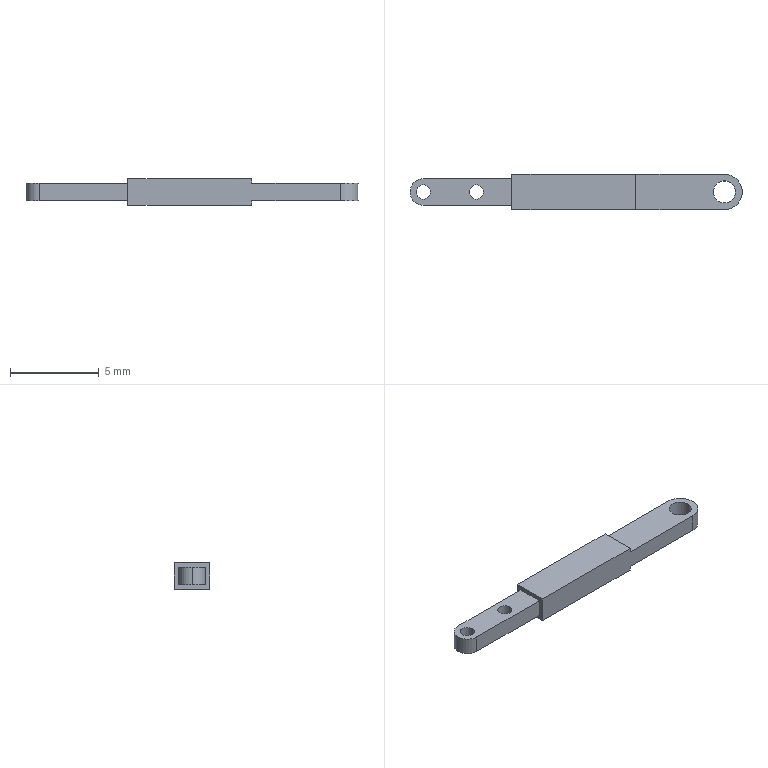Part | SolidWorks | features ICE 2, Extrusion 1, MirrorPattern 1 | 1 solid | 22 faces | box 18.75 x 2 x 1.5 mm | volume 38.722 mm3 | plane 13 | cylinder 9 | commonest cylinder face diameters 0.8 x4 1.25 x2 1.5 x2 2 x1
STEP:
#1=CARTESIAN_POINT('',(-2.4,0.,0.5));
#2=VERTEX_POINT('',#1);
#3=CARTESIAN_POINT('',(-1.6,0.,0.5));
#4=VERTEX_POINT('',#3);
#5=CARTESIAN_POINT('',(-2.,0.,0.5));
#6=DIRECTION('',(0.,0.,1.));
#7=DIRECTION('',(1.,0.,0.));
#8=AXIS2_PLACEMENT_3D('',#5,#6,#7);
#9=CIRCLE('',#8,0.4);
#10=EDGE_CURVE('',#2,#4,#9,.T.);
#11=ORIENTED_EDGE('',*,*,#10,.T.);
#12=CARTESIAN_POINT('',(-1.6,0.,-0.5));
#13=VERTEX_POINT('',#12);
#14=CARTESIAN_POINT('',(-1.6,0.,0.5));
#15=DIRECTION('',(0.,0.,-1.));
#16=VECTOR('',#15,1000.);
#17=LINE('',#14,#16);
#18=EDGE_CURVE('',#4,#13,#17,.T.);
#19=ORIENTED_EDGE('',*,*,#18,.T.);
#20=CARTESIAN_POINT('',(-2.4,0.,-0.5));
#21=VERTEX_POINT('',#20);
#22=CARTESIAN_POINT('',(-2.,0.,-0.5));
#23=DIRECTION('',(0.,0.,1.));
#24=DIRECTION('',(1.,0.,0.));
#25=AXIS2_PLACEMENT_3D('',#22,#23,#24);
#26=CIRCLE('',#25,0.4);
#27=EDGE_CURVE('',#21,#13,#26,.T.);
#28=ORIENTED_EDGE('',*,*,#27,.F.);
#29=CARTESIAN_POINT('',(-2.4,0.,0.5));
#30=DIRECTION('',(0.,0.,-1.));
#31=VECTOR('',#30,1000.);
#32=LINE('',#29,#31);
#33=EDGE_CURVE('',#2,#21,#32,.T.);
#34=ORIENTED_EDGE('',*,*,#33,.F.);
#35=EDGE_LOOP('',(#11,#19,#28,#34));
#36=FACE_OUTER_BOUND('',#35,.T.);
#37=CARTESIAN_POINT('',(-2.,0.,0.5));
#38=DIRECTION('',(0.,0.,-1.));
#39=DIRECTION('',(-1.,0.,0.));
#40=AXIS2_PLACEMENT_3D('',#37,#38,#39);
#41=CYLINDRICAL_SURFACE('',#40,0.4);
#42=ADVANCED_FACE('',(#36),#41,.F.);
#43=CARTESIAN_POINT('',(-5.4,0.,0.5));
#44=VERTEX_POINT('',#43);
#45=CARTESIAN_POINT('',(-4.6,0.,0.5));
#46=VERTEX_POINT('',#45);
#47=CARTESIAN_POINT('',(-5.,0.,0.5));
#48=DIRECTION('',(0.,0.,1.));
#49=DIRECTION('',(1.,0.,0.));
#50=AXIS2_PLACEMENT_3D('',#47,#48,#49);
#51=CIRCLE('',#50,0.4);
#52=EDGE_CURVE('',#44,#46,#51,.T.);
#53=ORIENTED_EDGE('',*,*,#52,.T.);
#54=CARTESIAN_POINT('',(-4.6,0.,-0.5));
#55=VERTEX_POINT('',#54);
#56=CARTESIAN_POINT('',(-4.6,0.,0.5));
#57=DIRECTION('',(0.,0.,-1.));
#58=VECTOR('',#57,1000.);
#59=LINE('',#56,#58);
#60=EDGE_CURVE('',#46,#55,#59,.T.);
#61=ORIENTED_EDGE('',*,*,#60,.T.);
#62=CARTESIAN_POINT('',(-5.4,0.,-0.5));
#63=VERTEX_POINT('',#62);
#64=CARTESIAN_POINT('',(-5.,0.,-0.5));
#65=DIRECTION('',(0.,0.,1.));
#66=DIRECTION('',(1.,0.,0.));
#67=AXIS2_PLACEMENT_3D('',#64,#65,#66);
#68=CIRCLE('',#67,0.4);
#69=EDGE_CURVE('',#63,#55,#68,.T.);
#70=ORIENTED_EDGE('',*,*,#69,.F.);
#71=CARTESIAN_POINT('',(-5.4,0.,0.5));
#72=DIRECTION('',(0.,0.,-1.));
#73=VECTOR('',#72,1000.);
#74=LINE('',#71,#73);
#75=EDGE_CURVE('',#44,#63,#74,.T.);
#76=ORIENTED_EDGE('',*,*,#75,.F.);
#77=EDGE_LOOP('',(#53,#61,#70,#76));
#78=FACE_OUTER_BOUND('',#77,.T.);
#79=CARTESIAN_POINT('',(-5.,0.,0.5));
#80=DIRECTION('',(0.,0.,-1.));
#81=DIRECTION('',(-1.,0.,0.));
#82=AXIS2_PLACEMENT_3D('',#79,#80,#81);
#83=CYLINDRICAL_SURFACE('',#82,0.4);
#84=ADVANCED_FACE('',(#78),#83,.F.);
#85=CARTESIAN_POINT('',(-5.75,0.,0.5));
#86=VERTEX_POINT('',#85);
#87=CARTESIAN_POINT('',(-5.,-0.75,0.5));
#88=VERTEX_POINT('',#87);
#89=CARTESIAN_POINT('',(-5.,0.,0.5));
#90=DIRECTION('',(0.,0.,1.));
#91=DIRECTION('',(-1.,0.,0.));
#92=AXIS2_PLACEMENT_3D('',#89,#90,#91);
#93=CIRCLE('',#92,0.75);
#94=EDGE_CURVE('',#86,#88,#93,.T.);
#95=ORIENTED_EDGE('',*,*,#94,.F.);
#96=CARTESIAN_POINT('',(-5.75,0.,-0.5));
#97=VERTEX_POINT('',#96);
#98=CARTESIAN_POINT('',(-5.75,0.,0.5));
#99=DIRECTION('',(0.,0.,-1.));
#100=VECTOR('',#99,1000.);
#101=LINE('',#98,#100);
#102=EDGE_CURVE('',#86,#97,#101,.T.);
#103=ORIENTED_EDGE('',*,*,#102,.T.);
#104=CARTESIAN_POINT('',(-5.,-0.75,-0.5));
#105=VERTEX_POINT('',#104);
#106=CARTESIAN_POINT('',(-5.,0.,-0.5));
#107=DIRECTION('',(0.,0.,1.));
#108=DIRECTION('',(-1.,0.,0.));
#109=AXIS2_PLACEMENT_3D('',#106,#107,#108);
#110=CIRCLE('',#109,0.75);
#111=EDGE_CURVE('',#97,#105,#110,.T.);
#112=ORIENTED_EDGE('',*,*,#111,.T.);
#113=CARTESIAN_POINT('',(-5.,-0.75,0.5));
#114=DIRECTION('',(0.,0.,-1.));
#115=VECTOR('',#114,1000.);
#116=LINE('',#113,#115);
#117=EDGE_CURVE('',#88,#105,#116,.T.);
#118=ORIENTED_EDGE('',*,*,#117,.F.);
#119=EDGE_LOOP('',(#95,#103,#112,#118));
#120=FACE_OUTER_BOUND('',#119,.T.);
#121=CARTESIAN_POINT('',(-5.,0.,0.5));
#122=DIRECTION('',(0.,0.,-1.));
#123=DIRECTION('',(-1.,0.,0.));
#124=AXIS2_PLACEMENT_3D('',#121,#122,#123);
#125=CYLINDRICAL_SURFACE('',#124,0.75);
#126=ADVANCED_FACE('',(#120),#125,.T.);
#127=CARTESIAN_POINT('',(12.625,0.,0.5));
#128=VERTEX_POINT('',#127);
#129=CARTESIAN_POINT('',(11.375,0.,0.5));
#130=VERTEX_POINT('',#129);
#131=CARTESIAN_POINT('',(12.,0.,0.5));
#132=DIRECTION('',(0.,0.,-1.));
#133=DIRECTION('',(-1.,0.,0.));
#134=AXIS2_PLACEMENT_3D('',#131,#132,#133);
#135=CIRCLE('',#134,0.625);
#136=EDGE_CURVE('',#128,#130,#135,.T.);
#137=ORIENTED_EDGE('',*,*,#136,.F.);
#138=CARTESIAN_POINT('',(12.625,0.,-0.5));
#139=VERTEX_POINT('',#138);
#140=CARTESIAN_POINT('',(12.625,0.,0.75));
#141=DIRECTION('',(0.,0.,-1.));
#142=VECTOR('',#141,1000.);
#143=LINE('',#140,#142);
#144=EDGE_CURVE('',#128,#139,#143,.T.);
#145=ORIENTED_EDGE('',*,*,#144,.T.);
#146=CARTESIAN_POINT('',(11.375,0.,-0.5));
#147=VERTEX_POINT('',#146);
#148=CARTESIAN_POINT('',(12.,0.,-0.5));
#149=DIRECTION('',(0.,0.,1.));
#150=DIRECTION('',(1.,0.,0.));
#151=AXIS2_PLACEMENT_3D('',#148,#149,#150);
#152=CIRCLE('',#151,0.625);
#153=EDGE_CURVE('',#147,#139,#152,.T.);
#154=ORIENTED_EDGE('',*,*,#153,.F.);
#155=CARTESIAN_POINT('',(11.375,0.,0.75));
#156=DIRECTION('',(0.,0.,-1.));
#157=VECTOR('',#156,1000.);
#158=LINE('',#155,#157);
#159=EDGE_CURVE('',#130,#147,#158,.T.);
#160=ORIENTED_EDGE('',*,*,#159,.F.);
#161=EDGE_LOOP('',(#137,#145,#154,#160));
#162=FACE_OUTER_BOUND('',#161,.T.);
#163=CARTESIAN_POINT('',(12.,0.,0.75));
#164=DIRECTION('',(0.,0.,-1.));
#165=DIRECTION('',(-1.,0.,0.));
#166=AXIS2_PLACEMENT_3D('',#163,#164,#165);
#167=CYLINDRICAL_SURFACE('',#166,0.625);
#168=ADVANCED_FACE('',(#162),#167,.F.);
#169=CARTESIAN_POINT('',(7.,-1.,0.75));
#170=VERTEX_POINT('',#169);
#171=CARTESIAN_POINT('',(7.,1.,0.75));
#172=VERTEX_POINT('',#171);
#173=CARTESIAN_POINT('',(7.,1.,0.75));
#174=DIRECTION('',(0.,1.,0.));
#175=VECTOR('',#174,1000.);
#176=LINE('',#173,#175);
#177=EDGE_CURVE('',#170,#172,#176,.T.);
#178=ORIENTED_EDGE('',*,*,#177,.T.);
#179=CARTESIAN_POINT('',(0.,1.,0.75));
#180=VERTEX_POINT('',#179);
#181=CARTESIAN_POINT('',(0.,1.,0.75));
#182=DIRECTION('',(-1.,0.,0.));
#183=VECTOR('',#182,1000.);
#184=LINE('',#181,#183);
#185=EDGE_CURVE('',#172,#180,#184,.T.);
#186=ORIENTED_EDGE('',*,*,#185,.T.);
#187=CARTESIAN_POINT('',(0.,-1.,0.75));
#188=VERTEX_POINT('',#187);
#189=CARTESIAN_POINT('',(0.,-1.,0.75));
#190=DIRECTION('',(0.,-1.,0.));
#191=VECTOR('',#190,1000.);
#192=LINE('',#189,#191);
#193=EDGE_CURVE('',#180,#188,#192,.T.);
#194=ORIENTED_EDGE('',*,*,#193,.T.);
#195=CARTESIAN_POINT('',(12.,-1.,0.75));
#196=DIRECTION('',(1.,0.,0.));
#197=VECTOR('',#196,1000.);
#198=LINE('',#195,#197);
#199=EDGE_CURVE('',#188,#170,#198,.T.);
#200=ORIENTED_EDGE('',*,*,#199,.T.);
#201=EDGE_LOOP('',(#178,#186,#194,#200));
#202=FACE_OUTER_BOUND('',#201,.T.);
#203=CARTESIAN_POINT('',(12.,0.,0.75));
#204=DIRECTION('',(0.,0.,-1.));
#205=DIRECTION('',(-1.,0.,0.));
#206=AXIS2_PLACEMENT_3D('',#203,#204,#205);
#207=PLANE('',#206);
#208=ADVANCED_FACE('',(#202),#207,.F.);
#209=CARTESIAN_POINT('',(7.,-1.,0.5));
#210=VERTEX_POINT('',#209);
#211=CARTESIAN_POINT('',(7.,-1.,0.5));
#212=DIRECTION('',(0.,0.,1.));
#213=VECTOR('',#212,1000.);
#214=LINE('',#211,#213);
#215=EDGE_CURVE('',#210,#170,#214,.T.);
#216=ORIENTED_EDGE('',*,*,#215,.T.);
#217=ORIENTED_EDGE('',*,*,#199,.F.);
#218=CARTESIAN_POINT('',(0.,-1.,-0.75));
#219=VERTEX_POINT('',#218);
#220=CARTESIAN_POINT('',(0.,-1.,0.75));
#221=DIRECTION('',(0.,0.,-1.));
#222=VECTOR('',#221,1000.);
#223=LINE('',#220,#222);
#224=EDGE_CURVE('',#188,#219,#223,.T.);
#225=ORIENTED_EDGE('',*,*,#224,.T.);
#226=CARTESIAN_POINT('',(7.,-1.,-0.75));
#227=VERTEX_POINT('',#226);
#228=CARTESIAN_POINT('',(12.,-1.,-0.75));
#229=DIRECTION('',(1.,0.,0.));
#230=VECTOR('',#229,1000.);
#231=LINE('',#228,#230);
#232=EDGE_CURVE('',#219,#227,#231,.T.);
#233=ORIENTED_EDGE('',*,*,#232,.T.);
#234=CARTESIAN_POINT('',(7.,-1.,-0.5));
#235=VERTEX_POINT('',#234);
#236=CARTESIAN_POINT('',(7.,-1.,-0.5));
#237=DIRECTION('',(0.,0.,-1.));
#238=VECTOR('',#237,1000.);
#239=LINE('',#236,#238);
#240=EDGE_CURVE('',#235,#227,#239,.T.);
#241=ORIENTED_EDGE('',*,*,#240,.F.);
#242=CARTESIAN_POINT('',(12.,-1.,-0.5));
#243=VERTEX_POINT('',#242);
#244=CARTESIAN_POINT('',(7.,-1.,-0.5));
#245=DIRECTION('',(-1.,0.,0.));
#246=VECTOR('',#245,1000.);
#247=LINE('',#244,#246);
#248=EDGE_CURVE('',#243,#235,#247,.T.);
#249=ORIENTED_EDGE('',*,*,#248,.F.);
#250=CARTESIAN_POINT('',(12.,-1.,0.5));
#251=VERTEX_POINT('',#250);
#252=CARTESIAN_POINT('',(12.,-1.,0.75));
#253=DIRECTION('',(0.,0.,-1.));
#254=VECTOR('',#253,1000.);
#255=LINE('',#252,#254);
#256=EDGE_CURVE('',#251,#243,#255,.T.);
#257=ORIENTED_EDGE('',*,*,#256,.F.);
#258=CARTESIAN_POINT('',(7.,-1.,0.5));
#259=DIRECTION('',(-1.,0.,0.));
#260=VECTOR('',#259,1000.);
#261=LINE('',#258,#260);
#262=EDGE_CURVE('',#251,#210,#261,.T.);
#263=ORIENTED_EDGE('',*,*,#262,.T.);
#264=EDGE_LOOP('',(#216,#217,#225,#233,#241,#249,#257,#263));
#265=FACE_OUTER_BOUND('',#264,.T.);
#266=CARTESIAN_POINT('',(12.,-1.,0.75));
#267=DIRECTION('',(0.,1.,0.));
#268=DIRECTION('',(-1.,0.,0.));
#269=AXIS2_PLACEMENT_3D('',#266,#267,#268);
#270=PLANE('',#269);
#271=ADVANCED_FACE('',(#265),#270,.F.);
#272=CARTESIAN_POINT('',(7.,1.,0.5));
#273=VERTEX_POINT('',#272);
#274=CARTESIAN_POINT('',(7.,1.,0.5));
#275=DIRECTION('',(0.,0.,1.));
#276=VECTOR('',#275,1000.);
#277=LINE('',#274,#276);
#278=EDGE_CURVE('',#273,#172,#277,.T.);
#279=ORIENTED_EDGE('',*,*,#278,.F.);
#280=CARTESIAN_POINT('',(12.,1.,0.5));
#281=VERTEX_POINT('',#280);
#282=CARTESIAN_POINT('',(12.,1.,0.5));
#283=DIRECTION('',(1.,0.,0.));
#284=VECTOR('',#283,1000.);
#285=LINE('',#282,#284);
#286=EDGE_CURVE('',#273,#281,#285,.T.);
#287=ORIENTED_EDGE('',*,*,#286,.T.);
#288=CARTESIAN_POINT('',(12.,1.,-0.5));
#289=VERTEX_POINT('',#288);
#290=CARTESIAN_POINT('',(12.,1.,0.75));
#291=DIRECTION('',(0.,0.,-1.));
#292=VECTOR('',#291,1000.);
#293=LINE('',#290,#292);
#294=EDGE_CURVE('',#281,#289,#293,.T.);
#295=ORIENTED_EDGE('',*,*,#294,.T.);
#296=CARTESIAN_POINT('',(7.,1.,-0.5));
#297=VERTEX_POINT('',#296);
#298=CARTESIAN_POINT('',(12.,1.,-0.5));
#299=DIRECTION('',(1.,0.,0.));
#300=VECTOR('',#299,1000.);
#301=LINE('',#298,#300);
#302=EDGE_CURVE('',#297,#289,#301,.T.);
#303=ORIENTED_EDGE('',*,*,#302,.F.);
#304=CARTESIAN_POINT('',(7.,1.,-0.75));
#305=VERTEX_POINT('',#304);
#306=CARTESIAN_POINT('',(7.,1.,-0.5));
#307=DIRECTION('',(0.,0.,-1.));
#308=VECTOR('',#307,1000.);
#309=LINE('',#306,#308);
#310=EDGE_CURVE('',#297,#305,#309,.T.);
#311=ORIENTED_EDGE('',*,*,#310,.T.);
#312=CARTESIAN_POINT('',(0.,1.,-0.75));
#313=VERTEX_POINT('',#312);
#314=CARTESIAN_POINT('',(0.,1.,-0.75));
#315=DIRECTION('',(-1.,0.,0.));
#316=VECTOR('',#315,1000.);
#317=LINE('',#314,#316);
#318=EDGE_CURVE('',#305,#313,#317,.T.);
#319=ORIENTED_EDGE('',*,*,#318,.T.);
#320=CARTESIAN_POINT('',(0.,1.,0.75));
#321=DIRECTION('',(0.,0.,-1.));
#322=VECTOR('',#321,1000.);
#323=LINE('',#320,#322);
#324=EDGE_CURVE('',#180,#313,#323,.T.);
#325=ORIENTED_EDGE('',*,*,#324,.F.);
#326=ORIENTED_EDGE('',*,*,#185,.F.);
#327=EDGE_LOOP('',(#279,#287,#295,#303,#311,#319,#325,#326));
#328=FACE_OUTER_BOUND('',#327,.T.);
#329=CARTESIAN_POINT('',(0.,1.,0.75));
#330=DIRECTION('',(0.,-1.,0.));
#331=DIRECTION('',(1.,0.,0.));
#332=AXIS2_PLACEMENT_3D('',#329,#330,#331);
#333=PLANE('',#332);
#334=ADVANCED_FACE('',(#328),#333,.F.);
#335=CARTESIAN_POINT('',(7.,1.,-0.75));
#336=DIRECTION('',(0.,1.,0.));
#337=VECTOR('',#336,1000.);
#338=LINE('',#335,#337);
#339=EDGE_CURVE('',#227,#305,#338,.T.);
#340=ORIENTED_EDGE('',*,*,#339,.F.);
#341=ORIENTED_EDGE('',*,*,#232,.F.);
#342=CARTESIAN_POINT('',(0.,-1.,-0.75));
#343=DIRECTION('',(0.,-1.,0.));
#344=VECTOR('',#343,1000.);
#345=LINE('',#342,#344);
#346=EDGE_CURVE('',#313,#219,#345,.T.);
#347=ORIENTED_EDGE('',*,*,#346,.F.);
#348=ORIENTED_EDGE('',*,*,#318,.F.);
#349=EDGE_LOOP('',(#340,#341,#347,#348));
#350=FACE_OUTER_BOUND('',#349,.T.);
#351=CARTESIAN_POINT('',(12.,0.,-0.75));
#352=DIRECTION('',(0.,0.,-1.));
#353=DIRECTION('',(-1.,0.,0.));
#354=AXIS2_PLACEMENT_3D('',#351,#352,#353);
#355=PLANE('',#354);
#356=ADVANCED_FACE('',(#350),#355,.T.);
#357=ORIENTED_EDGE('',*,*,#294,.F.);
#358=CARTESIAN_POINT('',(12.,0.,0.5));
#359=DIRECTION('',(0.,0.,-1.));
#360=DIRECTION('',(1.,0.,0.));
#361=AXIS2_PLACEMENT_3D('',#358,#359,#360);
#362=CIRCLE('',#361,1.);
#363=EDGE_CURVE('',#281,#251,#362,.T.);
#364=ORIENTED_EDGE('',*,*,#363,.T.);
#365=ORIENTED_EDGE('',*,*,#256,.T.);
#366=CARTESIAN_POINT('',(12.,0.,-0.5));
#367=DIRECTION('',(0.,0.,-1.));
#368=DIRECTION('',(1.,0.,0.));
#369=AXIS2_PLACEMENT_3D('',#366,#367,#368);
#370=CIRCLE('',#369,1.);
#371=EDGE_CURVE('',#289,#243,#370,.T.);
#372=ORIENTED_EDGE('',*,*,#371,.F.);
#373=EDGE_LOOP('',(#357,#364,#365,#372));
#374=FACE_OUTER_BOUND('',#373,.T.);
#375=CARTESIAN_POINT('',(12.,0.,0.75));
#376=DIRECTION('',(0.,0.,-1.));
#377=DIRECTION('',(-1.,0.,0.));
#378=AXIS2_PLACEMENT_3D('',#375,#376,#377);
#379=CYLINDRICAL_SURFACE('',#378,1.);
#380=ADVANCED_FACE('',(#374),#379,.T.);
#381=CARTESIAN_POINT('',(0.,-0.75,0.5));
#382=VERTEX_POINT('',#381);
#383=CARTESIAN_POINT('',(0.,-0.75,-0.5));
#384=VERTEX_POINT('',#383);
#385=CARTESIAN_POINT('',(0.,-0.75,0.5));
#386=DIRECTION('',(0.,0.,-1.));
#387=VECTOR('',#386,1000.);
#388=LINE('',#385,#387);
#389=EDGE_CURVE('',#382,#384,#388,.T.);
#390=ORIENTED_EDGE('',*,*,#389,.T.);
#391=CARTESIAN_POINT('',(0.,0.75,-0.5));
#392=VERTEX_POINT('',#391);
#393=CARTESIAN_POINT('',(0.,0.75,-0.5));
#394=DIRECTION('',(0.,1.,0.));
#395=VECTOR('',#394,1000.);
#396=LINE('',#393,#395);
#397=EDGE_CURVE('',#384,#392,#396,.T.);
#398=ORIENTED_EDGE('',*,*,#397,.T.);
#399=CARTESIAN_POINT('',(0.,0.75,0.5));
#400=VERTEX_POINT('',#399);
#401=CARTESIAN_POINT('',(0.,0.75,0.5));
#402=DIRECTION('',(0.,0.,-1.));
#403=VECTOR('',#402,1000.);
#404=LINE('',#401,#403);
#405=EDGE_CURVE('',#400,#392,#404,.T.);
#406=ORIENTED_EDGE('',*,*,#405,.F.);
#407=CARTESIAN_POINT('',(0.,0.75,0.5));
#408=DIRECTION('',(0.,1.,0.));
#409=VECTOR('',#408,1000.);
#410=LINE('',#407,#409);
#411=EDGE_CURVE('',#382,#400,#410,.T.);
#412=ORIENTED_EDGE('',*,*,#411,.F.);
#413=EDGE_LOOP('',(#390,#398,#406,#412));
#414=FACE_BOUND('',#413,.T.);
#415=ORIENTED_EDGE('',*,*,#346,.T.);
#416=ORIENTED_EDGE('',*,*,#224,.F.);
#417=ORIENTED_EDGE('',*,*,#193,.F.);
#418=ORIENTED_EDGE('',*,*,#324,.T.);
#419=EDGE_LOOP('',(#415,#416,#417,#418));
#420=FACE_OUTER_BOUND('',#419,.T.);
#421=CARTESIAN_POINT('',(0.,-1.,0.75));
#422=DIRECTION('',(1.,0.,0.));
#423=DIRECTION('',(0.,0.,-1.));
#424=AXIS2_PLACEMENT_3D('',#421,#422,#423);
#425=PLANE('',#424);
#426=ADVANCED_FACE('',(#414,#420),#425,.F.);
#427=ORIENTED_EDGE('',*,*,#144,.F.);
#428=CARTESIAN_POINT('',(12.,0.,0.5));
#429=DIRECTION('',(0.,0.,-1.));
#430=DIRECTION('',(-1.,0.,0.));
#431=AXIS2_PLACEMENT_3D('',#428,#429,#430);
#432=CIRCLE('',#431,0.625);
#433=EDGE_CURVE('',#130,#128,#432,.T.);
#434=ORIENTED_EDGE('',*,*,#433,.F.);
#435=ORIENTED_EDGE('',*,*,#159,.T.);
#436=CARTESIAN_POINT('',(12.,0.,-0.5));
#437=DIRECTION('',(0.,0.,1.));
#438=DIRECTION('',(1.,0.,0.));
#439=AXIS2_PLACEMENT_3D('',#436,#437,#438);
#440=CIRCLE('',#439,0.625);
#441=EDGE_CURVE('',#139,#147,#440,.T.);
#442=ORIENTED_EDGE('',*,*,#441,.F.);
#443=EDGE_LOOP('',(#427,#434,#435,#442));
#444=FACE_OUTER_BOUND('',#443,.T.);
#445=CARTESIAN_POINT('',(12.,0.,0.75));
#446=DIRECTION('',(0.,0.,-1.));
#447=DIRECTION('',(-1.,0.,0.));
#448=AXIS2_PLACEMENT_3D('',#445,#446,#447);
#449=CYLINDRICAL_SURFACE('',#448,0.625);
#450=ADVANCED_FACE('',(#444),#449,.F.);
#451=ORIENTED_EDGE('',*,*,#411,.T.);
#452=CARTESIAN_POINT('',(-5.,0.75,0.5));
#453=VERTEX_POINT('',#452);
#454=CARTESIAN_POINT('',(0.,0.75,0.5));
#455=DIRECTION('',(-1.,0.,0.));
#456=VECTOR('',#455,1000.);
#457=LINE('',#454,#456);
#458=EDGE_CURVE('',#400,#453,#457,.T.);
#459=ORIENTED_EDGE('',*,*,#458,.T.);
#460=CARTESIAN_POINT('',(-5.,0.,0.5));
#461=DIRECTION('',(0.,0.,1.));
#462=DIRECTION('',(-1.,0.,0.));
#463=AXIS2_PLACEMENT_3D('',#460,#461,#462);
#464=CIRCLE('',#463,0.75);
#465=EDGE_CURVE('',#453,#86,#464,.T.);
#466=ORIENTED_EDGE('',*,*,#465,.T.);
#467=ORIENTED_EDGE('',*,*,#94,.T.);
#468=CARTESIAN_POINT('',(0.,-0.75,0.5));
#469=DIRECTION('',(1.,0.,0.));
#470=VECTOR('',#469,1000.);
#471=LINE('',#468,#470);
#472=EDGE_CURVE('',#88,#382,#471,.T.);
#473=ORIENTED_EDGE('',*,*,#472,.T.);
#474=EDGE_LOOP('',(#451,#459,#466,#467,#473));
#475=FACE_OUTER_BOUND('',#474,.T.);
#476=ORIENTED_EDGE('',*,*,#52,.F.);
#477=CARTESIAN_POINT('',(-5.,0.,0.5));
#478=DIRECTION('',(0.,0.,1.));
#479=DIRECTION('',(1.,0.,0.));
#480=AXIS2_PLACEMENT_3D('',#477,#478,#479);
#481=CIRCLE('',#480,0.4);
#482=EDGE_CURVE('',#46,#44,#481,.T.);
#483=ORIENTED_EDGE('',*,*,#482,.F.);
#484=EDGE_LOOP('',(#476,#483));
#485=FACE_BOUND('',#484,.T.);
#486=ORIENTED_EDGE('',*,*,#10,.F.);
#487=CARTESIAN_POINT('',(-2.,0.,0.5));
#488=DIRECTION('',(0.,0.,1.));
#489=DIRECTION('',(1.,0.,0.));
#490=AXIS2_PLACEMENT_3D('',#487,#488,#489);
#491=CIRCLE('',#490,0.4);
#492=EDGE_CURVE('',#4,#2,#491,.T.);
#493=ORIENTED_EDGE('',*,*,#492,.F.);
#494=EDGE_LOOP('',(#486,#493));
#495=FACE_BOUND('',#494,.T.);
#496=CARTESIAN_POINT('',(-5.,0.,0.5));
#497=DIRECTION('',(0.,0.,-1.));
#498=DIRECTION('',(-1.,0.,0.));
#499=AXIS2_PLACEMENT_3D('',#496,#497,#498);
#500=PLANE('',#499);
#501=ADVANCED_FACE('',(#475,#485,#495),#500,.F.);
#502=ORIENTED_EDGE('',*,*,#69,.T.);
#503=CARTESIAN_POINT('',(-5.,0.,-0.5));
#504=DIRECTION('',(0.,0.,1.));
#505=DIRECTION('',(1.,0.,0.));
#506=AXIS2_PLACEMENT_3D('',#503,#504,#505);
#507=CIRCLE('',#506,0.4);
#508=EDGE_CURVE('',#55,#63,#507,.T.);
#509=ORIENTED_EDGE('',*,*,#508,.T.);
#510=EDGE_LOOP('',(#502,#509));
#511=FACE_BOUND('',#510,.T.);
#512=ORIENTED_EDGE('',*,*,#397,.F.);
#513=CARTESIAN_POINT('',(0.,-0.75,-0.5));
#514=DIRECTION('',(1.,0.,0.));
#515=VECTOR('',#514,1000.);
#516=LINE('',#513,#515);
#517=EDGE_CURVE('',#105,#384,#516,.T.);
#518=ORIENTED_EDGE('',*,*,#517,.F.);
#519=ORIENTED_EDGE('',*,*,#111,.F.);
#520=CARTESIAN_POINT('',(-5.,0.75,-0.5));
#521=VERTEX_POINT('',#520);
#522=CARTESIAN_POINT('',(-5.,0.,-0.5));
#523=DIRECTION('',(0.,0.,1.));
#524=DIRECTION('',(-1.,0.,0.));
#525=AXIS2_PLACEMENT_3D('',#522,#523,#524);
#526=CIRCLE('',#525,0.75);
#527=EDGE_CURVE('',#521,#97,#526,.T.);
#528=ORIENTED_EDGE('',*,*,#527,.F.);
#529=CARTESIAN_POINT('',(0.,0.75,-0.5));
#530=DIRECTION('',(-1.,0.,0.));
#531=VECTOR('',#530,1000.);
#532=LINE('',#529,#531);
#533=EDGE_CURVE('',#392,#521,#532,.T.);
#534=ORIENTED_EDGE('',*,*,#533,.F.);
#535=EDGE_LOOP('',(#512,#518,#519,#528,#534));
#536=FACE_OUTER_BOUND('',#535,.T.);
#537=ORIENTED_EDGE('',*,*,#27,.T.);
#538=CARTESIAN_POINT('',(-2.,0.,-0.5));
#539=DIRECTION('',(0.,0.,1.));
#540=DIRECTION('',(1.,0.,0.));
#541=AXIS2_PLACEMENT_3D('',#538,#539,#540);
#542=CIRCLE('',#541,0.4);
#543=EDGE_CURVE('',#13,#21,#542,.T.);
#544=ORIENTED_EDGE('',*,*,#543,.T.);
#545=EDGE_LOOP('',(#537,#544));
#546=FACE_BOUND('',#545,.T.);
#547=CARTESIAN_POINT('',(-5.,0.,-0.5));
#548=DIRECTION('',(0.,0.,-1.));
#549=DIRECTION('',(-1.,0.,0.));
#550=AXIS2_PLACEMENT_3D('',#547,#548,#549);
#551=PLANE('',#550);
#552=ADVANCED_FACE('',(#511,#536,#546),#551,.T.);
#553=ORIENTED_EDGE('',*,*,#533,.T.);
#554=CARTESIAN_POINT('',(-5.,0.75,0.5));
#555=DIRECTION('',(0.,0.,-1.));
#556=VECTOR('',#555,1000.);
#557=LINE('',#554,#556);
#558=EDGE_CURVE('',#453,#521,#557,.T.);
#559=ORIENTED_EDGE('',*,*,#558,.F.);
#560=ORIENTED_EDGE('',*,*,#458,.F.);
#561=ORIENTED_EDGE('',*,*,#405,.T.);
#562=EDGE_LOOP('',(#553,#559,#560,#561));
#563=FACE_OUTER_BOUND('',#562,.T.);
#564=CARTESIAN_POINT('',(0.,0.75,0.5));
#565=DIRECTION('',(0.,-1.,0.));
#566=DIRECTION('',(1.,0.,0.));
#567=AXIS2_PLACEMENT_3D('',#564,#565,#566);
#568=PLANE('',#567);
#569=ADVANCED_FACE('',(#563),#568,.F.);
#570=ORIENTED_EDGE('',*,*,#102,.F.);
#571=ORIENTED_EDGE('',*,*,#465,.F.);
#572=ORIENTED_EDGE('',*,*,#558,.T.);
#573=ORIENTED_EDGE('',*,*,#527,.T.);
#574=EDGE_LOOP('',(#570,#571,#572,#573));
#575=FACE_OUTER_BOUND('',#574,.T.);
#576=CARTESIAN_POINT('',(-5.,0.,0.5));
#577=DIRECTION('',(0.,0.,-1.));
#578=DIRECTION('',(-1.,0.,0.));
#579=AXIS2_PLACEMENT_3D('',#576,#577,#578);
#580=CYLINDRICAL_SURFACE('',#579,0.75);
#581=ADVANCED_FACE('',(#575),#580,.T.);
#582=ORIENTED_EDGE('',*,*,#517,.T.);
#583=ORIENTED_EDGE('',*,*,#389,.F.);
#584=ORIENTED_EDGE('',*,*,#472,.F.);
#585=ORIENTED_EDGE('',*,*,#117,.T.);
#586=EDGE_LOOP('',(#582,#583,#584,#585));
#587=FACE_OUTER_BOUND('',#586,.T.);
#588=CARTESIAN_POINT('',(0.,-0.75,0.5));
#589=DIRECTION('',(0.,1.,0.));
#590=DIRECTION('',(-1.,0.,0.));
#591=AXIS2_PLACEMENT_3D('',#588,#589,#590);
#592=PLANE('',#591);
#593=ADVANCED_FACE('',(#587),#592,.F.);
#594=ORIENTED_EDGE('',*,*,#60,.F.);
#595=ORIENTED_EDGE('',*,*,#482,.T.);
#596=ORIENTED_EDGE('',*,*,#75,.T.);
#597=ORIENTED_EDGE('',*,*,#508,.F.);
#598=EDGE_LOOP('',(#594,#595,#596,#597));
#599=FACE_OUTER_BOUND('',#598,.T.);
#600=CARTESIAN_POINT('',(-5.,0.,0.5));
#601=DIRECTION('',(0.,0.,-1.));
#602=DIRECTION('',(-1.,0.,0.));
#603=AXIS2_PLACEMENT_3D('',#600,#601,#602);
#604=CYLINDRICAL_SURFACE('',#603,0.4);
#605=ADVANCED_FACE('',(#599),#604,.F.);
#606=ORIENTED_EDGE('',*,*,#18,.F.);
#607=ORIENTED_EDGE('',*,*,#492,.T.);
#608=ORIENTED_EDGE('',*,*,#33,.T.);
#609=ORIENTED_EDGE('',*,*,#543,.F.);
#610=EDGE_LOOP('',(#606,#607,#608,#609));
#611=FACE_OUTER_BOUND('',#610,.T.);
#612=CARTESIAN_POINT('',(-2.,0.,0.5));
#613=DIRECTION('',(0.,0.,-1.));
#614=DIRECTION('',(-1.,0.,0.));
#615=AXIS2_PLACEMENT_3D('',#612,#613,#614);
#616=CYLINDRICAL_SURFACE('',#615,0.4);
#617=ADVANCED_FACE('',(#611),#616,.F.);
#618=ORIENTED_EDGE('',*,*,#339,.T.);
#619=ORIENTED_EDGE('',*,*,#310,.F.);
#620=CARTESIAN_POINT('',(7.,1.,-0.5));
#621=DIRECTION('',(0.,1.,0.));
#622=VECTOR('',#621,1000.);
#623=LINE('',#620,#622);
#624=EDGE_CURVE('',#235,#297,#623,.T.);
#625=ORIENTED_EDGE('',*,*,#624,.F.);
#626=ORIENTED_EDGE('',*,*,#240,.T.);
#627=EDGE_LOOP('',(#618,#619,#625,#626));
#628=FACE_OUTER_BOUND('',#627,.T.);
#629=CARTESIAN_POINT('',(7.,1.,-0.5));
#630=DIRECTION('',(-1.,0.,0.));
#631=DIRECTION('',(0.,0.,1.));
#632=AXIS2_PLACEMENT_3D('',#629,#630,#631);
#633=PLANE('',#632);
#634=ADVANCED_FACE('',(#628),#633,.F.);
#635=ORIENTED_EDGE('',*,*,#153,.T.);
#636=ORIENTED_EDGE('',*,*,#441,.T.);
#637=EDGE_LOOP('',(#635,#636));
#638=FACE_BOUND('',#637,.T.);
#639=ORIENTED_EDGE('',*,*,#302,.T.);
#640=ORIENTED_EDGE('',*,*,#371,.T.);
#641=ORIENTED_EDGE('',*,*,#248,.T.);
#642=ORIENTED_EDGE('',*,*,#624,.T.);
#643=EDGE_LOOP('',(#639,#640,#641,#642));
#644=FACE_OUTER_BOUND('',#643,.T.);
#645=CARTESIAN_POINT('',(12.,0.,-0.5));
#646=DIRECTION('',(0.,0.,1.));
#647=DIRECTION('',(1.,0.,0.));
#648=AXIS2_PLACEMENT_3D('',#645,#646,#647);
#649=PLANE('',#648);
#650=ADVANCED_FACE('',(#638,#644),#649,.F.);
#651=ORIENTED_EDGE('',*,*,#177,.F.);
#652=ORIENTED_EDGE('',*,*,#215,.F.);
#653=CARTESIAN_POINT('',(7.,1.,0.5));
#654=DIRECTION('',(0.,1.,0.));
#655=VECTOR('',#654,1000.);
#656=LINE('',#653,#655);
#657=EDGE_CURVE('',#210,#273,#656,.T.);
#658=ORIENTED_EDGE('',*,*,#657,.T.);
#659=ORIENTED_EDGE('',*,*,#278,.T.);
#660=EDGE_LOOP('',(#651,#652,#658,#659));
#661=FACE_OUTER_BOUND('',#660,.T.);
#662=CARTESIAN_POINT('',(7.,1.,0.5));
#663=DIRECTION('',(1.,0.,0.));
#664=DIRECTION('',(0.,0.,-1.));
#665=AXIS2_PLACEMENT_3D('',#662,#663,#664);
#666=PLANE('',#665);
#667=ADVANCED_FACE('',(#661),#666,.T.);
#668=ORIENTED_EDGE('',*,*,#433,.T.);
#669=ORIENTED_EDGE('',*,*,#136,.T.);
#670=EDGE_LOOP('',(#668,#669));
#671=FACE_BOUND('',#670,.T.);
#672=ORIENTED_EDGE('',*,*,#286,.F.);
#673=ORIENTED_EDGE('',*,*,#657,.F.);
#674=ORIENTED_EDGE('',*,*,#262,.F.);
#675=ORIENTED_EDGE('',*,*,#363,.F.);
#676=EDGE_LOOP('',(#672,#673,#674,#675));
#677=FACE_OUTER_BOUND('',#676,.T.);
#678=CARTESIAN_POINT('',(12.,0.,0.5));
#679=DIRECTION('',(0.,0.,-1.));
#680=DIRECTION('',(1.,0.,0.));
#681=AXIS2_PLACEMENT_3D('',#678,#679,#680);
#682=PLANE('',#681);
#683=ADVANCED_FACE('',(#671,#677),#682,.F.);
#684=CLOSED_SHELL('',(#42,#84,#126,#168,#208,#271,#334,#356,#380,#426,#450,#501,#552,#569,#581,#593,#605,#617,#634,#650,#667,#683));
#685=MANIFOLD_SOLID_BREP('',#684);
#686=CARTESIAN_POINT('',(0.,0.,0.));
#687=DIRECTION('',(0.,0.,1.));
#688=DIRECTION('',(1.,0.,0.));
#689=AXIS2_PLACEMENT_3D('',#686,#687,#688);
#690=(LENGTH_UNIT()NAMED_UNIT(*)SI_UNIT(.MILLI.,.METRE.));
#691=UNCERTAINTY_MEASURE_WITH_UNIT(LENGTH_MEASURE(0.00001),#690,'','');
#692=(NAMED_UNIT(*)PLANE_ANGLE_UNIT()SI_UNIT($,.RADIAN.));
#693=(NAMED_UNIT(*)SI_UNIT($,.STERADIAN.)SOLID_ANGLE_UNIT());
#694=(GEOMETRIC_REPRESENTATION_CONTEXT(3)GLOBAL_UNCERTAINTY_ASSIGNED_CONTEXT((#691))GLOBAL_UNIT_ASSIGNED_CONTEXT((#690,#692,#693))REPRESENTATION_CONTEXT('',''));
#695=ADVANCED_BREP_SHAPE_REPRESENTATION('',(#685,#689),#694);